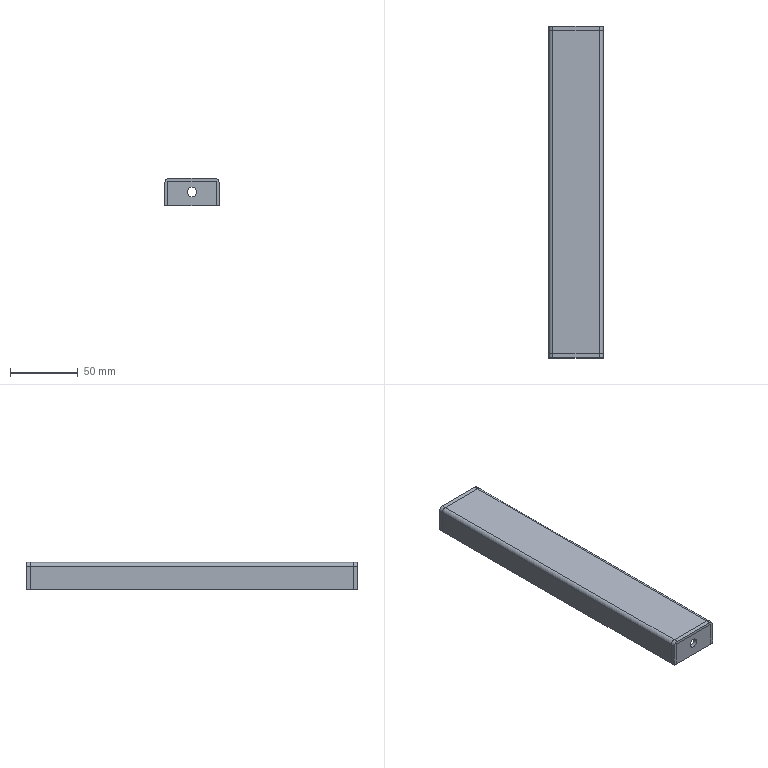Part | STEP file | MM-P46715-05_1 | 3 solids | 34 faces | box 40 x 245 x 20 mm | volume 40958 mm3 | plane 22 | cylinder 12 | commonest cylinder face diameters 6 x6 6.8 x4 2 x2